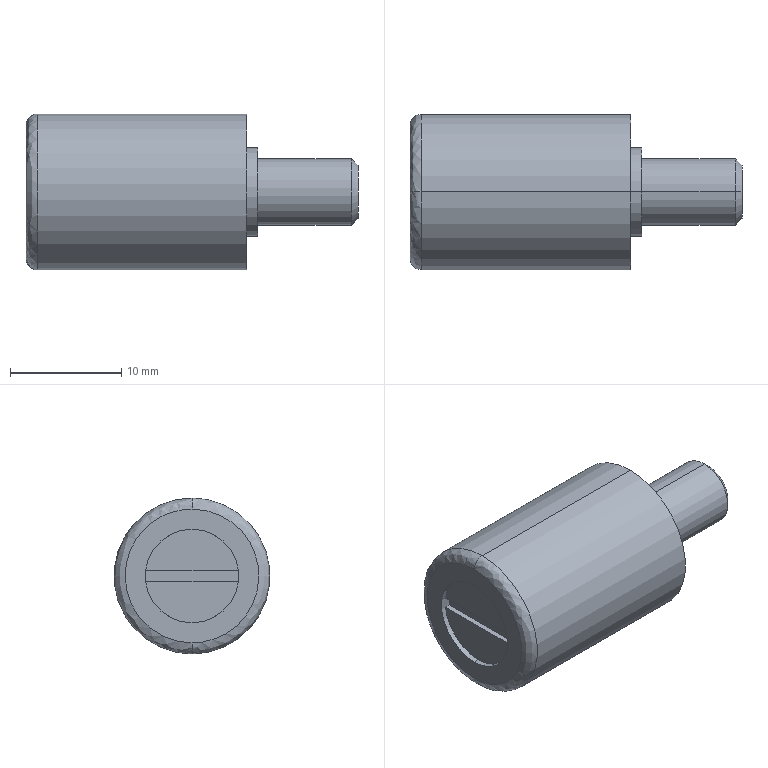Part | STEP file | 0232_Z_HOKW63_2 | 1 solid | 21 faces | box 29.8 x 14 x 14 mm | volume 3308 mm3 | plane 9 | cylinder 8 | spline 2 | cone 2 | commonest cylinder face diameters 6 x2 8 x2 8.4 x2 14 x2